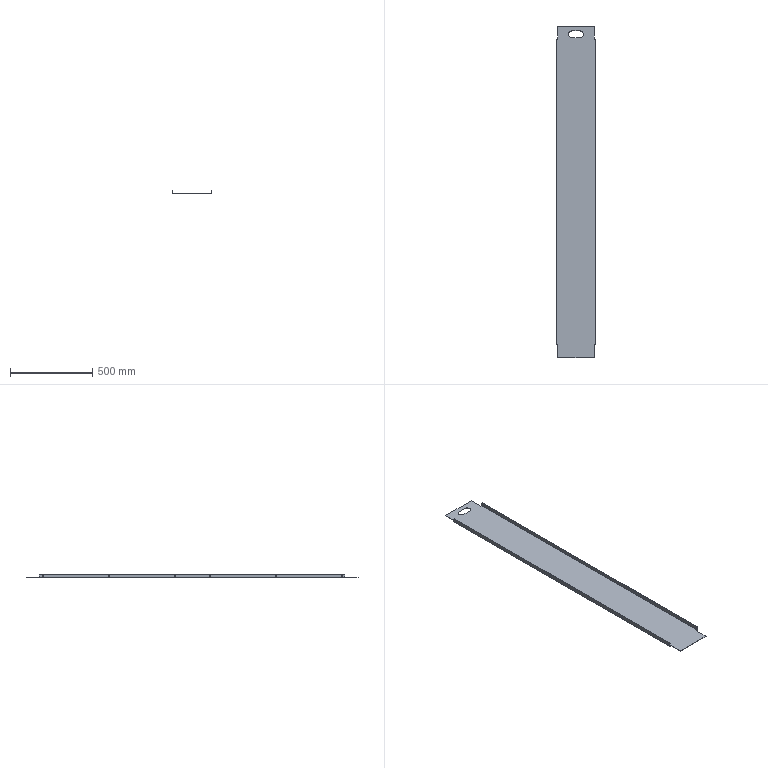Part | 1 solid | 65 faces | box 240 x 2016 x 23 mm | volume 832892 mm3 | plane 34 | cylinder 31 | commonest cylinder face diameters 6.2 x24 40 x3 0.4 x2 3.4 x2